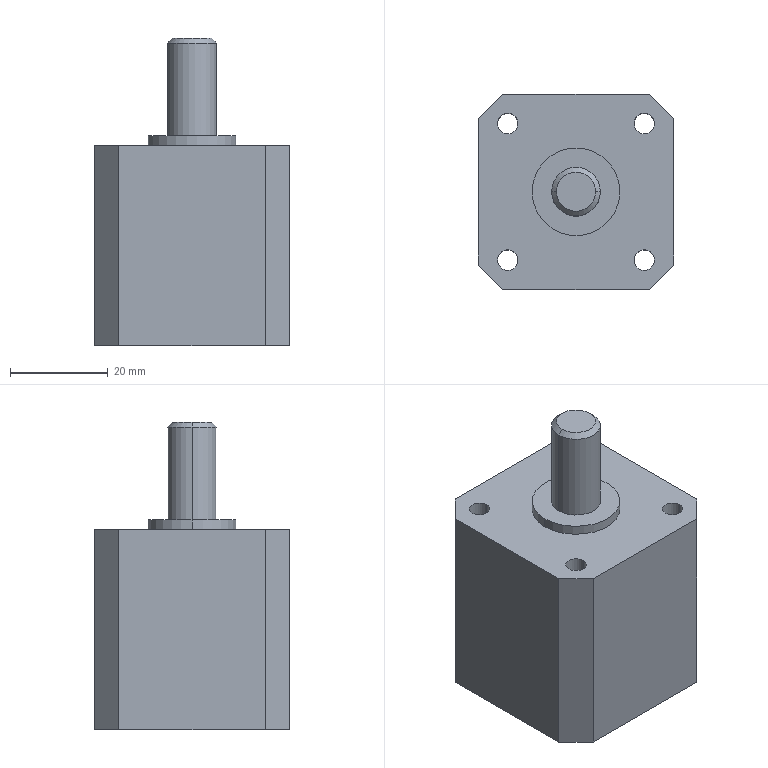Part | 1 solid | 255 faces | box 40 x 40 x 63 mm | volume 63343 mm3 | plane 139 | spline 102 | cylinder 12 | cone 2 | commonest cylinder face diameters 4.2 x8 10 x2 18 x2